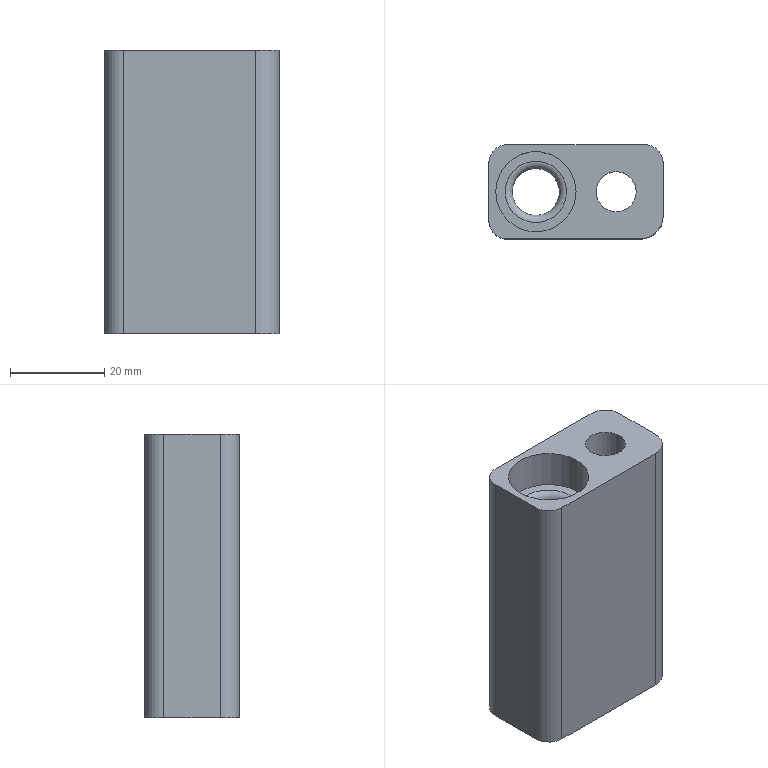Part | STEP file | gslz 2016.10.28-10_id662_x_t | 1 solid | 17 faces | box 37 x 20 x 60 mm | volume 30244 mm3 | plane 8 | cylinder 8 | torus 1 | commonest cylinder face diameters 8 x3 10 x2 8.5 x1 14 x1 17 x1
STEP:
#1=CARTESIAN_POINT('',(0.,0.,0.));
#2=DIRECTION('',(0.,0.,1.));
#3=DIRECTION('',(1.,0.,0.));
#4=AXIS2_PLACEMENT_3D('',#1,#2,#3);
#5=CARTESIAN_POINT('',(1137.841,70.167,85.));
#6=VERTEX_POINT('',#5);
#7=CARTESIAN_POINT('',(1146.341,70.167,85.));
#8=DIRECTION('',(0.,0.,1.));
#9=DIRECTION('',(-1.,0.,0.));
#10=AXIS2_PLACEMENT_3D('',#7,#8,#9);
#11=CIRCLE('',#10,8.5);
#12=CARTESIAN_POINT('',(1105.341,76.167,85.));
#13=DIRECTION('',(0.,0.,1.));
#14=DIRECTION('',(1.,0.,0.));
#15=AXIS2_PLACEMENT_3D('',#12,#13,#14);
#16=PLANE('',#15);
#17=CARTESIAN_POINT('',(41.,-6.));
#18=DIRECTION('',(-1.,0.));
#19=AXIS2_PLACEMENT_2D('',#17,#18);
#20=CIRCLE('',#19,8.5);
#21=(GEOMETRIC_REPRESENTATION_CONTEXT(2)PARAMETRIC_REPRESENTATION_CONTEXT()REPRESENTATION_CONTEXT('',''));
#22=DEFINITIONAL_REPRESENTATION('',(#20),#21);
#23=PCURVE('',#16,#22);
#24=CARTESIAN_POINT('',(1146.341,70.167,81.));
#25=DIRECTION('',(0.,0.,-1.));
#26=DIRECTION('',(1.,0.,0.));
#27=AXIS2_PLACEMENT_3D('',#24,#25,#26);
#28=CYLINDRICAL_SURFACE('',#27,8.5);
#29=CARTESIAN_POINT('',(9.425,-4.));
#30=DIRECTION('',(-1.,0.));
#31=VECTOR('',#30,1.);
#32=LINE('',#29,#31);
#33=(GEOMETRIC_REPRESENTATION_CONTEXT(2)PARAMETRIC_REPRESENTATION_CONTEXT()REPRESENTATION_CONTEXT('',''));
#34=DEFINITIONAL_REPRESENTATION('',(#32),#33);
#35=PCURVE('',#28,#34);
#36=SURFACE_CURVE('',#11,(#23,#35),.PCURVE_S1.);
#37=EDGE_CURVE('',#6,#6,#36,.T.);
#38=ORIENTED_EDGE('',*,*,#37,.F.);
#39=EDGE_LOOP('',(#38));
#40=FACE_BOUND('',#39,.T.);
#41=CARTESIAN_POINT('',(1173.341,65.167,85.));
#42=VERTEX_POINT('',#41);
#43=CARTESIAN_POINT('',(1173.341,76.167,85.));
#44=VERTEX_POINT('',#43);
#45=CARTESIAN_POINT('',(1173.341,76.167,85.));
#46=DIRECTION('',(0.,1.,0.));
#47=VECTOR('',#46,1.);
#48=LINE('',#45,#47);
#49=CARTESIAN_POINT('',(68.,0.));
#50=DIRECTION('',(0.,1.));
#51=VECTOR('',#50,1.);
#52=LINE('',#49,#51);
#53=(GEOMETRIC_REPRESENTATION_CONTEXT(2)PARAMETRIC_REPRESENTATION_CONTEXT()REPRESENTATION_CONTEXT('',''));
#54=DEFINITIONAL_REPRESENTATION('',(#52),#53);
#55=PCURVE('',#16,#54);
#56=CARTESIAN_POINT('',(1173.341,70.167,43.5));
#57=DIRECTION('',(1.,0.,0.));
#58=DIRECTION('',(0.,0.,-1.));
#59=AXIS2_PLACEMENT_3D('',#56,#57,#58);
#60=PLANE('',#59);
#61=CARTESIAN_POINT('',(-41.5,6.));
#62=DIRECTION('',(0.,1.));
#63=VECTOR('',#62,1.);
#64=LINE('',#61,#63);
#65=(GEOMETRIC_REPRESENTATION_CONTEXT(2)PARAMETRIC_REPRESENTATION_CONTEXT()REPRESENTATION_CONTEXT('',''));
#66=DEFINITIONAL_REPRESENTATION('',(#64),#65);
#67=PCURVE('',#60,#66);
#68=SURFACE_CURVE('',#48,(#55,#67),.PCURVE_S1.);
#69=EDGE_CURVE('',#42,#44,#68,.T.);
#70=ORIENTED_EDGE('',*,*,#69,.T.);
#71=CARTESIAN_POINT('',(1169.341,80.167,85.));
#72=VERTEX_POINT('',#71);
#73=CARTESIAN_POINT('',(1169.341,76.167,85.));
#74=DIRECTION('',(0.,0.,1.));
#75=DIRECTION('',(-1.,0.,0.));
#76=AXIS2_PLACEMENT_3D('',#73,#74,#75);
#77=CIRCLE('',#76,4.);
#78=CARTESIAN_POINT('',(64.,0.));
#79=DIRECTION('',(-1.,0.));
#80=AXIS2_PLACEMENT_2D('',#78,#79);
#81=CIRCLE('',#80,4.);
#82=(GEOMETRIC_REPRESENTATION_CONTEXT(2)PARAMETRIC_REPRESENTATION_CONTEXT()REPRESENTATION_CONTEXT('',''));
#83=DEFINITIONAL_REPRESENTATION('',(#81),#82);
#84=PCURVE('',#16,#83);
#85=CARTESIAN_POINT('',(1169.341,76.167,43.5));
#86=DIRECTION('',(0.,0.,-1.));
#87=DIRECTION('',(-1.,0.,0.));
#88=AXIS2_PLACEMENT_3D('',#85,#86,#87);
#89=CYLINDRICAL_SURFACE('',#88,4.);
#90=CARTESIAN_POINT('',(6.283,-41.5));
#91=DIRECTION('',(-1.,0.));
#92=VECTOR('',#91,1.);
#93=LINE('',#90,#92);
#94=(GEOMETRIC_REPRESENTATION_CONTEXT(2)PARAMETRIC_REPRESENTATION_CONTEXT()REPRESENTATION_CONTEXT('',''));
#95=DEFINITIONAL_REPRESENTATION('',(#93),#94);
#96=PCURVE('',#89,#95);
#97=SURFACE_CURVE('',#77,(#84,#96),.PCURVE_S1.);
#98=EDGE_CURVE('',#44,#72,#97,.T.);
#99=ORIENTED_EDGE('',*,*,#98,.T.);
#100=CARTESIAN_POINT('',(1140.341,80.167,85.));
#101=VERTEX_POINT('',#100);
#102=CARTESIAN_POINT('',(1062.706,80.167,85.));
#103=DIRECTION('',(-1.,0.,0.));
#104=VECTOR('',#103,1.);
#105=LINE('',#102,#104);
#106=CARTESIAN_POINT('',(-42.635,4.));
#107=DIRECTION('',(-1.,0.));
#108=VECTOR('',#107,1.);
#109=LINE('',#106,#108);
#110=(GEOMETRIC_REPRESENTATION_CONTEXT(2)PARAMETRIC_REPRESENTATION_CONTEXT()REPRESENTATION_CONTEXT('',''));
#111=DEFINITIONAL_REPRESENTATION('',(#109),#110);
#112=PCURVE('',#16,#111);
#113=CARTESIAN_POINT('',(1062.706,80.167,80.));
#114=DIRECTION('',(0.,-1.,0.));
#115=DIRECTION('',(0.,0.,-1.));
#116=AXIS2_PLACEMENT_3D('',#113,#114,#115);
#117=PLANE('',#116);
#118=CARTESIAN_POINT('',(-5.,0.));
#119=DIRECTION('',(0.,-1.));
#120=VECTOR('',#119,1.);
#121=LINE('',#118,#120);
#122=(GEOMETRIC_REPRESENTATION_CONTEXT(2)PARAMETRIC_REPRESENTATION_CONTEXT()REPRESENTATION_CONTEXT('',''));
#123=DEFINITIONAL_REPRESENTATION('',(#121),#122);
#124=PCURVE('',#117,#123);
#125=SURFACE_CURVE('',#105,(#112,#124),.PCURVE_S1.);
#126=EDGE_CURVE('',#72,#101,#125,.T.);
#127=ORIENTED_EDGE('',*,*,#126,.T.);
#128=CARTESIAN_POINT('',(1136.341,76.167,85.));
#129=VERTEX_POINT('',#128);
#130=CARTESIAN_POINT('',(1140.341,76.167,85.));
#131=DIRECTION('',(0.,0.,1.));
#132=DIRECTION('',(-1.,0.,0.));
#133=AXIS2_PLACEMENT_3D('',#130,#131,#132);
#134=CIRCLE('',#133,4.);
#135=CARTESIAN_POINT('',(35.,0.));
#136=DIRECTION('',(-1.,0.));
#137=AXIS2_PLACEMENT_2D('',#135,#136);
#138=CIRCLE('',#137,4.);
#139=(GEOMETRIC_REPRESENTATION_CONTEXT(2)PARAMETRIC_REPRESENTATION_CONTEXT()REPRESENTATION_CONTEXT('',''));
#140=DEFINITIONAL_REPRESENTATION('',(#138),#139);
#141=PCURVE('',#16,#140);
#142=CARTESIAN_POINT('',(1140.341,76.167,46.));
#143=DIRECTION('',(0.,0.,-1.));
#144=DIRECTION('',(-1.,0.,0.));
#145=AXIS2_PLACEMENT_3D('',#142,#143,#144);
#146=CYLINDRICAL_SURFACE('',#145,4.);
#147=CARTESIAN_POINT('',(6.283,-39.));
#148=DIRECTION('',(-1.,0.));
#149=VECTOR('',#148,1.);
#150=LINE('',#147,#149);
#151=(GEOMETRIC_REPRESENTATION_CONTEXT(2)PARAMETRIC_REPRESENTATION_CONTEXT()REPRESENTATION_CONTEXT('',''));
#152=DEFINITIONAL_REPRESENTATION('',(#150),#151);
#153=PCURVE('',#146,#152);
#154=SURFACE_CURVE('',#134,(#141,#153),.PCURVE_S1.);
#155=EDGE_CURVE('',#101,#129,#154,.T.);
#156=ORIENTED_EDGE('',*,*,#155,.T.);
#157=CARTESIAN_POINT('',(1136.341,64.167,85.));
#158=VERTEX_POINT('',#157);
#159=CARTESIAN_POINT('',(1136.341,70.167,85.));
#160=DIRECTION('',(0.,-1.,0.));
#161=VECTOR('',#160,1.);
#162=LINE('',#159,#161);
#163=CARTESIAN_POINT('',(31.,-6.));
#164=DIRECTION('',(0.,-1.));
#165=VECTOR('',#164,1.);
#166=LINE('',#163,#165);
#167=(GEOMETRIC_REPRESENTATION_CONTEXT(2)PARAMETRIC_REPRESENTATION_CONTEXT()REPRESENTATION_CONTEXT('',''));
#168=DEFINITIONAL_REPRESENTATION('',(#166),#167);
#169=PCURVE('',#16,#168);
#170=CARTESIAN_POINT('',(1136.341,70.167,46.));
#171=DIRECTION('',(1.,0.,0.));
#172=DIRECTION('',(0.,0.,-1.));
#173=AXIS2_PLACEMENT_3D('',#170,#171,#172);
#174=PLANE('',#173);
#175=CARTESIAN_POINT('',(-39.,0.));
#176=DIRECTION('',(0.,-1.));
#177=VECTOR('',#176,1.);
#178=LINE('',#175,#177);
#179=(GEOMETRIC_REPRESENTATION_CONTEXT(2)PARAMETRIC_REPRESENTATION_CONTEXT()REPRESENTATION_CONTEXT('',''));
#180=DEFINITIONAL_REPRESENTATION('',(#178),#179);
#181=PCURVE('',#174,#180);
#182=SURFACE_CURVE('',#162,(#169,#181),.PCURVE_S1.);
#183=EDGE_CURVE('',#129,#158,#182,.T.);
#184=ORIENTED_EDGE('',*,*,#183,.T.);
#185=CARTESIAN_POINT('',(1140.341,60.167,85.));
#186=VERTEX_POINT('',#185);
#187=CARTESIAN_POINT('',(1140.341,64.167,85.));
#188=DIRECTION('',(0.,0.,1.));
#189=DIRECTION('',(-1.,0.,0.));
#190=AXIS2_PLACEMENT_3D('',#187,#188,#189);
#191=CIRCLE('',#190,4.);
#192=CARTESIAN_POINT('',(35.,-12.));
#193=DIRECTION('',(-1.,0.));
#194=AXIS2_PLACEMENT_2D('',#192,#193);
#195=CIRCLE('',#194,4.);
#196=(GEOMETRIC_REPRESENTATION_CONTEXT(2)PARAMETRIC_REPRESENTATION_CONTEXT()REPRESENTATION_CONTEXT('',''));
#197=DEFINITIONAL_REPRESENTATION('',(#195),#196);
#198=PCURVE('',#16,#197);
#199=CARTESIAN_POINT('',(1140.341,64.167,80.));
#200=DIRECTION('',(0.,0.,-1.));
#201=DIRECTION('',(-1.,0.,0.));
#202=AXIS2_PLACEMENT_3D('',#199,#200,#201);
#203=CYLINDRICAL_SURFACE('',#202,4.);
#204=CARTESIAN_POINT('',(6.283,-5.));
#205=DIRECTION('',(-1.,0.));
#206=VECTOR('',#205,1.);
#207=LINE('',#204,#206);
#208=(GEOMETRIC_REPRESENTATION_CONTEXT(2)PARAMETRIC_REPRESENTATION_CONTEXT()REPRESENTATION_CONTEXT('',''));
#209=DEFINITIONAL_REPRESENTATION('',(#207),#208);
#210=PCURVE('',#203,#209);
#211=SURFACE_CURVE('',#191,(#198,#210),.PCURVE_S1.);
#212=EDGE_CURVE('',#158,#186,#211,.T.);
#213=ORIENTED_EDGE('',*,*,#212,.T.);
#214=CARTESIAN_POINT('',(1168.341,60.167,85.));
#215=VERTEX_POINT('',#214);
#216=CARTESIAN_POINT('',(1798.341,60.167,85.));
#217=DIRECTION('',(1.,0.,0.));
#218=VECTOR('',#217,1.);
#219=LINE('',#216,#218);
#220=CARTESIAN_POINT('',(693.,-16.));
#221=DIRECTION('',(1.,0.));
#222=VECTOR('',#221,1.);
#223=LINE('',#220,#222);
#224=(GEOMETRIC_REPRESENTATION_CONTEXT(2)PARAMETRIC_REPRESENTATION_CONTEXT()REPRESENTATION_CONTEXT('',''));
#225=DEFINITIONAL_REPRESENTATION('',(#223),#224);
#226=PCURVE('',#16,#225);
#227=CARTESIAN_POINT('',(1798.341,60.167,80.));
#228=DIRECTION('',(0.,1.,0.));
#229=DIRECTION('',(0.,0.,1.));
#230=AXIS2_PLACEMENT_3D('',#227,#228,#229);
#231=PLANE('',#230);
#232=CARTESIAN_POINT('',(5.,0.));
#233=DIRECTION('',(0.,1.));
#234=VECTOR('',#233,1.);
#235=LINE('',#232,#234);
#236=(GEOMETRIC_REPRESENTATION_CONTEXT(2)PARAMETRIC_REPRESENTATION_CONTEXT()REPRESENTATION_CONTEXT('',''));
#237=DEFINITIONAL_REPRESENTATION('',(#235),#236);
#238=PCURVE('',#231,#237);
#239=SURFACE_CURVE('',#219,(#226,#238),.PCURVE_S1.);
#240=EDGE_CURVE('',#186,#215,#239,.T.);
#241=ORIENTED_EDGE('',*,*,#240,.T.);
#242=CARTESIAN_POINT('',(1168.341,65.167,85.));
#243=DIRECTION('',(0.,0.,1.));
#244=DIRECTION('',(-1.,0.,0.));
#245=AXIS2_PLACEMENT_3D('',#242,#243,#244);
#246=CIRCLE('',#245,5.);
#247=CARTESIAN_POINT('',(63.,-11.));
#248=DIRECTION('',(-1.,0.));
#249=AXIS2_PLACEMENT_2D('',#247,#248);
#250=CIRCLE('',#249,5.);
#251=(GEOMETRIC_REPRESENTATION_CONTEXT(2)PARAMETRIC_REPRESENTATION_CONTEXT()REPRESENTATION_CONTEXT('',''));
#252=DEFINITIONAL_REPRESENTATION('',(#250),#251);
#253=PCURVE('',#16,#252);
#254=CARTESIAN_POINT('',(1168.341,65.167,43.5));
#255=DIRECTION('',(0.,0.,1.));
#256=DIRECTION('',(1.,0.,0.));
#257=AXIS2_PLACEMENT_3D('',#254,#255,#256);
#258=CYLINDRICAL_SURFACE('',#257,5.);
#259=CARTESIAN_POINT('',(3.142,41.5));
#260=DIRECTION('',(1.,0.));
#261=VECTOR('',#260,1.);
#262=LINE('',#259,#261);
#263=(GEOMETRIC_REPRESENTATION_CONTEXT(2)PARAMETRIC_REPRESENTATION_CONTEXT()REPRESENTATION_CONTEXT('',''));
#264=DEFINITIONAL_REPRESENTATION('',(#262),#263);
#265=PCURVE('',#258,#264);
#266=SURFACE_CURVE('',#246,(#253,#265),.PCURVE_S1.);
#267=EDGE_CURVE('',#215,#42,#266,.T.);
#268=ORIENTED_EDGE('',*,*,#267,.T.);
#269=EDGE_LOOP('',(#70,#99,#127,#156,#184,#213,#241,#268));
#270=FACE_BOUND('',#269,.T.);
#271=CARTESIAN_POINT('',(1159.091,70.167,85.));
#272=VERTEX_POINT('',#271);
#273=CARTESIAN_POINT('',(1163.341,70.167,85.));
#274=DIRECTION('',(0.,0.,-1.));
#275=DIRECTION('',(-1.,0.,0.));
#276=AXIS2_PLACEMENT_3D('',#273,#274,#275);
#277=CIRCLE('',#276,4.25);
#278=CARTESIAN_POINT('',(53.75,-6.));
#279=CARTESIAN_POINT('',(53.75,1.361));
#280=CARTESIAN_POINT('',(60.125,-2.319));
#281=CARTESIAN_POINT('',(66.5,-6.));
#282=CARTESIAN_POINT('',(60.125,-9.681));
#283=CARTESIAN_POINT('',(53.75,-13.361));
#284=CARTESIAN_POINT('',(53.75,-6.));
#285=(BOUNDED_CURVE()B_SPLINE_CURVE(2,(#278,#279,#280,#281,#282,#283,#284),.UNSPECIFIED.,.T.,.F.)B_SPLINE_CURVE_WITH_KNOTS((1,2,2,2,2,1),(-2.094,0.,2.094,4.189,6.283,8.378),.UNSPECIFIED.)CURVE()GEOMETRIC_REPRESENTATION_ITEM()RATIONAL_B_SPLINE_CURVE((1.,0.5,1.,0.5,1.,0.5,1.))REPRESENTATION_ITEM(''));
#286=(GEOMETRIC_REPRESENTATION_CONTEXT(2)PARAMETRIC_REPRESENTATION_CONTEXT()REPRESENTATION_CONTEXT('',''));
#287=DEFINITIONAL_REPRESENTATION('',(#285),#286);
#288=PCURVE('',#16,#287);
#289=CARTESIAN_POINT('',(1163.341,70.167,-18.));
#290=DIRECTION('',(0.,0.,1.));
#291=DIRECTION('',(1.,0.,0.));
#292=AXIS2_PLACEMENT_3D('',#289,#290,#291);
#293=CYLINDRICAL_SURFACE('',#292,4.25);
#294=CARTESIAN_POINT('',(9.425,103.));
#295=DIRECTION('',(-1.,0.));
#296=VECTOR('',#295,1.);
#297=LINE('',#294,#296);
#298=(GEOMETRIC_REPRESENTATION_CONTEXT(2)PARAMETRIC_REPRESENTATION_CONTEXT()REPRESENTATION_CONTEXT('',''));
#299=DEFINITIONAL_REPRESENTATION('',(#297),#298);
#300=PCURVE('',#293,#299);
#301=SURFACE_CURVE('',#277,(#288,#300),.PCURVE_S1.);
#302=EDGE_CURVE('',#272,#272,#301,.T.);
#303=ORIENTED_EDGE('',*,*,#302,.T.);
#304=EDGE_LOOP('',(#303));
#305=FACE_BOUND('',#304,.T.);
#306=ADVANCED_FACE('',(#40,#270,#305),#16,.T.);
#307=CARTESIAN_POINT('',(1151.341,70.167,25.));
#308=VERTEX_POINT('',#307);
#309=CARTESIAN_POINT('',(1146.341,70.167,25.));
#310=DIRECTION('',(0.,0.,1.));
#311=DIRECTION('',(1.,0.,0.));
#312=AXIS2_PLACEMENT_3D('',#309,#310,#311);
#313=CIRCLE('',#312,5.);
#314=CARTESIAN_POINT('',(1097.341,16.167,25.));
#315=DIRECTION('',(0.,0.,-1.));
#316=DIRECTION('',(-1.,0.,0.));
#317=AXIS2_PLACEMENT_3D('',#314,#315,#316);
#318=PLANE('',#317);
#319=CARTESIAN_POINT('',(-54.,54.));
#320=CARTESIAN_POINT('',(-54.,62.66));
#321=CARTESIAN_POINT('',(-46.5,58.33));
#322=CARTESIAN_POINT('',(-39.,54.));
#323=CARTESIAN_POINT('',(-46.5,49.67));
#324=CARTESIAN_POINT('',(-54.,45.34));
#325=CARTESIAN_POINT('',(-54.,54.));
#326=(BOUNDED_CURVE()B_SPLINE_CURVE(2,(#319,#320,#321,#322,#323,#324,#325),.UNSPECIFIED.,.T.,.F.)B_SPLINE_CURVE_WITH_KNOTS((1,2,2,2,2,1),(-2.094,0.,2.094,4.189,6.283,8.378),.UNSPECIFIED.)CURVE()GEOMETRIC_REPRESENTATION_ITEM()RATIONAL_B_SPLINE_CURVE((1.,0.5,1.,0.5,1.,0.5,1.))REPRESENTATION_ITEM(''));
#327=(GEOMETRIC_REPRESENTATION_CONTEXT(2)PARAMETRIC_REPRESENTATION_CONTEXT()REPRESENTATION_CONTEXT('',''));
#328=DEFINITIONAL_REPRESENTATION('',(#326),#327);
#329=PCURVE('',#318,#328);
#330=CARTESIAN_POINT('',(1146.341,70.167,45.5));
#331=DIRECTION('',(0.,0.,-1.));
#332=DIRECTION('',(1.,0.,0.));
#333=AXIS2_PLACEMENT_3D('',#330,#331,#332);
#334=CYLINDRICAL_SURFACE('',#333,5.);
#335=CARTESIAN_POINT('',(6.283,20.5));
#336=DIRECTION('',(-1.,0.));
#337=VECTOR('',#336,1.);
#338=LINE('',#335,#337);
#339=(GEOMETRIC_REPRESENTATION_CONTEXT(2)PARAMETRIC_REPRESENTATION_CONTEXT()REPRESENTATION_CONTEXT('',''));
#340=DEFINITIONAL_REPRESENTATION('',(#338),#339);
#341=PCURVE('',#334,#340);
#342=SURFACE_CURVE('',#313,(#329,#341),.PCURVE_S1.);
#343=EDGE_CURVE('',#308,#308,#342,.T.);
#344=ORIENTED_EDGE('',*,*,#343,.T.);
#345=EDGE_LOOP('',(#344));
#346=FACE_BOUND('',#345,.T.);
#347=CARTESIAN_POINT('',(1170.341,70.167,25.));
#348=VERTEX_POINT('',#347);
#349=CARTESIAN_POINT('',(1163.341,70.167,25.));
#350=DIRECTION('',(0.,0.,1.));
#351=DIRECTION('',(1.,0.,0.));
#352=AXIS2_PLACEMENT_3D('',#349,#350,#351);
#353=CIRCLE('',#352,7.);
#354=CARTESIAN_POINT('',(-73.,54.));
#355=CARTESIAN_POINT('',(-73.,66.124));
#356=CARTESIAN_POINT('',(-62.5,60.062));
#357=CARTESIAN_POINT('',(-52.,54.));
#358=CARTESIAN_POINT('',(-62.5,47.938));
#359=CARTESIAN_POINT('',(-73.,41.876));
#360=CARTESIAN_POINT('',(-73.,54.));
#361=(BOUNDED_CURVE()B_SPLINE_CURVE(2,(#354,#355,#356,#357,#358,#359,#360),.UNSPECIFIED.,.T.,.F.)B_SPLINE_CURVE_WITH_KNOTS((1,2,2,2,2,1),(-2.094,0.,2.094,4.189,6.283,8.378),.UNSPECIFIED.)CURVE()GEOMETRIC_REPRESENTATION_ITEM()RATIONAL_B_SPLINE_CURVE((1.,0.5,1.,0.5,1.,0.5,1.))REPRESENTATION_ITEM(''));
#362=(GEOMETRIC_REPRESENTATION_CONTEXT(2)PARAMETRIC_REPRESENTATION_CONTEXT()REPRESENTATION_CONTEXT('',''));
#363=DEFINITIONAL_REPRESENTATION('',(#361),#362);
#364=PCURVE('',#318,#363);
#365=CARTESIAN_POINT('',(1163.341,70.167,-8.));
#366=DIRECTION('',(0.,0.,1.));
#367=DIRECTION('',(1.,0.,0.));
#368=AXIS2_PLACEMENT_3D('',#365,#366,#367);
#369=CYLINDRICAL_SURFACE('',#368,7.);
#370=CARTESIAN_POINT('',(0.,33.));
#371=DIRECTION('',(1.,0.));
#372=VECTOR('',#371,1.);
#373=LINE('',#370,#372);
#374=(GEOMETRIC_REPRESENTATION_CONTEXT(2)PARAMETRIC_REPRESENTATION_CONTEXT()REPRESENTATION_CONTEXT('',''));
#375=DEFINITIONAL_REPRESENTATION('',(#373),#374);
#376=PCURVE('',#369,#375);
#377=SURFACE_CURVE('',#353,(#364,#376),.PCURVE_S1.);
#378=EDGE_CURVE('',#348,#348,#377,.T.);
#379=ORIENTED_EDGE('',*,*,#378,.T.);
#380=EDGE_LOOP('',(#379));
#381=FACE_BOUND('',#380,.T.);
#382=CARTESIAN_POINT('',(1169.341,80.167,25.));
#383=VERTEX_POINT('',#382);
#384=CARTESIAN_POINT('',(1140.341,80.167,25.));
#385=VERTEX_POINT('',#384);
#386=CARTESIAN_POINT('',(1097.341,80.167,25.));
#387=DIRECTION('',(-1.,0.,0.));
#388=VECTOR('',#387,1.);
#389=LINE('',#386,#388);
#390=CARTESIAN_POINT('',(0.,64.));
#391=DIRECTION('',(1.,0.));
#392=VECTOR('',#391,1.);
#393=LINE('',#390,#392);
#394=(GEOMETRIC_REPRESENTATION_CONTEXT(2)PARAMETRIC_REPRESENTATION_CONTEXT()REPRESENTATION_CONTEXT('',''));
#395=DEFINITIONAL_REPRESENTATION('',(#393),#394);
#396=PCURVE('',#318,#395);
#397=CARTESIAN_POINT('',(55.,34.635));
#398=DIRECTION('',(0.,-1.));
#399=VECTOR('',#398,1.);
#400=LINE('',#397,#399);
#401=(GEOMETRIC_REPRESENTATION_CONTEXT(2)PARAMETRIC_REPRESENTATION_CONTEXT()REPRESENTATION_CONTEXT('',''));
#402=DEFINITIONAL_REPRESENTATION('',(#400),#401);
#403=PCURVE('',#117,#402);
#404=SURFACE_CURVE('',#389,(#396,#403),.PCURVE_S1.);
#405=EDGE_CURVE('',#383,#385,#404,.T.);
#406=ORIENTED_EDGE('',*,*,#405,.F.);
#407=CARTESIAN_POINT('',(1173.341,76.167,25.));
#408=VERTEX_POINT('',#407);
#409=CARTESIAN_POINT('',(1169.341,76.167,25.));
#410=DIRECTION('',(0.,0.,-1.));
#411=DIRECTION('',(1.,0.,0.));
#412=AXIS2_PLACEMENT_3D('',#409,#410,#411);
#413=CIRCLE('',#412,4.);
#414=CARTESIAN_POINT('',(-72.,60.));
#415=DIRECTION('',(-1.,0.));
#416=AXIS2_PLACEMENT_2D('',#414,#415);
#417=CIRCLE('',#416,4.);
#418=(GEOMETRIC_REPRESENTATION_CONTEXT(2)PARAMETRIC_REPRESENTATION_CONTEXT()REPRESENTATION_CONTEXT('',''));
#419=DEFINITIONAL_REPRESENTATION('',(#417),#418);
#420=PCURVE('',#318,#419);
#421=CARTESIAN_POINT('',(-3.142,18.5));
#422=DIRECTION('',(1.,0.));
#423=VECTOR('',#422,1.);
#424=LINE('',#421,#423);
#425=(GEOMETRIC_REPRESENTATION_CONTEXT(2)PARAMETRIC_REPRESENTATION_CONTEXT()REPRESENTATION_CONTEXT('',''));
#426=DEFINITIONAL_REPRESENTATION('',(#424),#425);
#427=PCURVE('',#89,#426);
#428=SURFACE_CURVE('',#413,(#420,#427),.PCURVE_S1.);
#429=EDGE_CURVE('',#383,#408,#428,.T.);
#430=ORIENTED_EDGE('',*,*,#429,.T.);
#431=CARTESIAN_POINT('',(1173.341,65.167,25.));
#432=VERTEX_POINT('',#431);
#433=CARTESIAN_POINT('',(1173.341,16.167,25.));
#434=DIRECTION('',(0.,-1.,0.));
#435=VECTOR('',#434,1.);
#436=LINE('',#433,#435);
#437=CARTESIAN_POINT('',(-76.,0.));
#438=DIRECTION('',(0.,-1.));
#439=VECTOR('',#438,1.);
#440=LINE('',#437,#439);
#441=(GEOMETRIC_REPRESENTATION_CONTEXT(2)PARAMETRIC_REPRESENTATION_CONTEXT()REPRESENTATION_CONTEXT('',''));
#442=DEFINITIONAL_REPRESENTATION('',(#440),#441);
#443=PCURVE('',#318,#442);
#444=CARTESIAN_POINT('',(18.5,-54.));
#445=DIRECTION('',(0.,-1.));
#446=VECTOR('',#445,1.);
#447=LINE('',#444,#446);
#448=(GEOMETRIC_REPRESENTATION_CONTEXT(2)PARAMETRIC_REPRESENTATION_CONTEXT()REPRESENTATION_CONTEXT('',''));
#449=DEFINITIONAL_REPRESENTATION('',(#447),#448);
#450=PCURVE('',#60,#449);
#451=SURFACE_CURVE('',#436,(#443,#450),.PCURVE_S1.);
#452=EDGE_CURVE('',#408,#432,#451,.T.);
#453=ORIENTED_EDGE('',*,*,#452,.T.);
#454=CARTESIAN_POINT('',(1168.341,60.167,25.));
#455=VERTEX_POINT('',#454);
#456=CARTESIAN_POINT('',(1168.341,65.167,25.));
#457=DIRECTION('',(0.,0.,-1.));
#458=DIRECTION('',(1.,0.,0.));
#459=AXIS2_PLACEMENT_3D('',#456,#457,#458);
#460=CIRCLE('',#459,5.);
#461=CARTESIAN_POINT('',(-71.,49.));
#462=DIRECTION('',(-1.,0.));
#463=AXIS2_PLACEMENT_2D('',#461,#462);
#464=CIRCLE('',#463,5.);
#465=(GEOMETRIC_REPRESENTATION_CONTEXT(2)PARAMETRIC_REPRESENTATION_CONTEXT()REPRESENTATION_CONTEXT('',''));
#466=DEFINITIONAL_REPRESENTATION('',(#464),#465);
#467=PCURVE('',#318,#466);
#468=CARTESIAN_POINT('',(6.283,-18.5));
#469=DIRECTION('',(-1.,0.));
#470=VECTOR('',#469,1.);
#471=LINE('',#468,#470);
#472=(GEOMETRIC_REPRESENTATION_CONTEXT(2)PARAMETRIC_REPRESENTATION_CONTEXT()REPRESENTATION_CONTEXT('',''));
#473=DEFINITIONAL_REPRESENTATION('',(#471),#472);
#474=PCURVE('',#258,#473);
#475=SURFACE_CURVE('',#460,(#467,#474),.PCURVE_S1.);
#476=EDGE_CURVE('',#432,#455,#475,.T.);
#477=ORIENTED_EDGE('',*,*,#476,.T.);
#478=CARTESIAN_POINT('',(1140.341,60.167,25.));
#479=VERTEX_POINT('',#478);
#480=CARTESIAN_POINT('',(1097.341,60.167,25.));
#481=DIRECTION('',(1.,0.,0.));
#482=VECTOR('',#481,1.);
#483=LINE('',#480,#482);
#484=CARTESIAN_POINT('',(0.,44.));
#485=DIRECTION('',(-1.,0.));
#486=VECTOR('',#485,1.);
#487=LINE('',#484,#486);
#488=(GEOMETRIC_REPRESENTATION_CONTEXT(2)PARAMETRIC_REPRESENTATION_CONTEXT()REPRESENTATION_CONTEXT('',''));
#489=DEFINITIONAL_REPRESENTATION('',(#487),#488);
#490=PCURVE('',#318,#489);
#491=CARTESIAN_POINT('',(-55.,-701.));
#492=DIRECTION('',(0.,1.));
#493=VECTOR('',#492,1.);
#494=LINE('',#491,#493);
#495=(GEOMETRIC_REPRESENTATION_CONTEXT(2)PARAMETRIC_REPRESENTATION_CONTEXT()REPRESENTATION_CONTEXT('',''));
#496=DEFINITIONAL_REPRESENTATION('',(#494),#495);
#497=PCURVE('',#231,#496);
#498=SURFACE_CURVE('',#483,(#490,#497),.PCURVE_S1.);
#499=EDGE_CURVE('',#479,#455,#498,.T.);
#500=ORIENTED_EDGE('',*,*,#499,.F.);
#501=CARTESIAN_POINT('',(1136.341,64.167,25.));
#502=VERTEX_POINT('',#501);
#503=CARTESIAN_POINT('',(1140.341,64.167,25.));
#504=DIRECTION('',(0.,0.,-1.));
#505=DIRECTION('',(1.,0.,0.));
#506=AXIS2_PLACEMENT_3D('',#503,#504,#505);
#507=CIRCLE('',#506,4.);
#508=CARTESIAN_POINT('',(-43.,48.));
#509=DIRECTION('',(-1.,0.));
#510=AXIS2_PLACEMENT_2D('',#508,#509);
#511=CIRCLE('',#510,4.);
#512=(GEOMETRIC_REPRESENTATION_CONTEXT(2)PARAMETRIC_REPRESENTATION_CONTEXT()REPRESENTATION_CONTEXT('',''));
#513=DEFINITIONAL_REPRESENTATION('',(#511),#512);
#514=PCURVE('',#318,#513);
#515=CARTESIAN_POINT('',(3.142,55.));
#516=DIRECTION('',(1.,0.));
#517=VECTOR('',#516,1.);
#518=LINE('',#515,#517);
#519=(GEOMETRIC_REPRESENTATION_CONTEXT(2)PARAMETRIC_REPRESENTATION_CONTEXT()REPRESENTATION_CONTEXT('',''));
#520=DEFINITIONAL_REPRESENTATION('',(#518),#519);
#521=PCURVE('',#203,#520);
#522=SURFACE_CURVE('',#507,(#514,#521),.PCURVE_S1.);
#523=EDGE_CURVE('',#479,#502,#522,.T.);
#524=ORIENTED_EDGE('',*,*,#523,.T.);
#525=CARTESIAN_POINT('',(1136.341,76.167,25.));
#526=VERTEX_POINT('',#525);
#527=CARTESIAN_POINT('',(1136.341,70.167,25.));
#528=DIRECTION('',(0.,1.,0.));
#529=VECTOR('',#528,1.);
#530=LINE('',#527,#529);
#531=CARTESIAN_POINT('',(-39.,54.));
#532=DIRECTION('',(0.,1.));
#533=VECTOR('',#532,1.);
#534=LINE('',#531,#533);
#535=(GEOMETRIC_REPRESENTATION_CONTEXT(2)PARAMETRIC_REPRESENTATION_CONTEXT()REPRESENTATION_CONTEXT('',''));
#536=DEFINITIONAL_REPRESENTATION('',(#534),#535);
#537=PCURVE('',#318,#536);
#538=CARTESIAN_POINT('',(21.,0.));
#539=DIRECTION('',(0.,1.));
#540=VECTOR('',#539,1.);
#541=LINE('',#538,#540);
#542=(GEOMETRIC_REPRESENTATION_CONTEXT(2)PARAMETRIC_REPRESENTATION_CONTEXT()REPRESENTATION_CONTEXT('',''));
#543=DEFINITIONAL_REPRESENTATION('',(#541),#542);
#544=PCURVE('',#174,#543);
#545=SURFACE_CURVE('',#530,(#537,#544),.PCURVE_S1.);
#546=EDGE_CURVE('',#502,#526,#545,.T.);
#547=ORIENTED_EDGE('',*,*,#546,.T.);
#548=CARTESIAN_POINT('',(1140.341,76.167,25.));
#549=DIRECTION('',(0.,0.,-1.));
#550=DIRECTION('',(1.,0.,0.));
#551=AXIS2_PLACEMENT_3D('',#548,#549,#550);
#552=CIRCLE('',#551,4.);
#553=CARTESIAN_POINT('',(-43.,60.));
#554=DIRECTION('',(-1.,0.));
#555=AXIS2_PLACEMENT_2D('',#553,#554);
#556=CIRCLE('',#555,4.);
#557=(GEOMETRIC_REPRESENTATION_CONTEXT(2)PARAMETRIC_REPRESENTATION_CONTEXT()REPRESENTATION_CONTEXT('',''));
#558=DEFINITIONAL_REPRESENTATION('',(#556),#557);
#559=PCURVE('',#318,#558);
#560=CARTESIAN_POINT('',(-3.142,21.));
#561=DIRECTION('',(1.,0.));
#562=VECTOR('',#561,1.);
#563=LINE('',#560,#562);
#564=(GEOMETRIC_REPRESENTATION_CONTEXT(2)PARAMETRIC_REPRESENTATION_CONTEXT()REPRESENTATION_CONTEXT('',''));
#565=DEFINITIONAL_REPRESENTATION('',(#563),#564);
#566=PCURVE('',#146,#565);
#567=SURFACE_CURVE('',#552,(#559,#566),.PCURVE_S1.);
#568=EDGE_CURVE('',#526,#385,#567,.T.);
#569=ORIENTED_EDGE('',*,*,#568,.T.);
#570=EDGE_LOOP('',(#406,#430,#453,#477,#500,#524,#547,#569));
#571=FACE_BOUND('',#570,.T.);
#572=ADVANCED_FACE('',(#346,#381,#571),#318,.T.);
#573=ORIENTED_EDGE('',*,*,#499,.T.);
#574=CARTESIAN_POINT('',(1168.341,60.167,95.));
#575=DIRECTION('',(0.,0.,1.));
#576=VECTOR('',#575,1.);
#577=LINE('',#574,#576);
#578=CARTESIAN_POINT('',(15.,-630.));
#579=DIRECTION('',(1.,0.));
#580=VECTOR('',#579,1.);
#581=LINE('',#578,#580);
#582=(GEOMETRIC_REPRESENTATION_CONTEXT(2)PARAMETRIC_REPRESENTATION_CONTEXT()REPRESENTATION_CONTEXT('',''));
#583=DEFINITIONAL_REPRESENTATION('',(#581),#582);
#584=PCURVE('',#231,#583);
#585=CARTESIAN_POINT('',(4.712,51.5));
#586=DIRECTION('',(0.,1.));
#587=VECTOR('',#586,1.);
#588=LINE('',#585,#587);
#589=(GEOMETRIC_REPRESENTATION_CONTEXT(2)PARAMETRIC_REPRESENTATION_CONTEXT()REPRESENTATION_CONTEXT('',''));
#590=DEFINITIONAL_REPRESENTATION('',(#588),#589);
#591=PCURVE('',#258,#590);
#592=SURFACE_CURVE('',#577,(#584,#591),.PCURVE_S1.);
#593=EDGE_CURVE('',#455,#215,#592,.T.);
#594=ORIENTED_EDGE('',*,*,#593,.T.);
#595=ORIENTED_EDGE('',*,*,#240,.F.);
#596=CARTESIAN_POINT('',(1140.341,60.167,80.));
#597=DIRECTION('',(0.,0.,-1.));
#598=VECTOR('',#597,1.);
#599=LINE('',#596,#598);
#600=CARTESIAN_POINT('',(0.,-658.));
#601=DIRECTION('',(-1.,0.));
#602=VECTOR('',#601,1.);
#603=LINE('',#600,#602);
#604=(GEOMETRIC_REPRESENTATION_CONTEXT(2)PARAMETRIC_REPRESENTATION_CONTEXT()REPRESENTATION_CONTEXT('',''));
#605=DEFINITIONAL_REPRESENTATION('',(#603),#604);
#606=PCURVE('',#231,#605);
#607=CARTESIAN_POINT('',(4.712,0.));
#608=DIRECTION('',(0.,1.));
#609=VECTOR('',#608,1.);
#610=LINE('',#607,#609);
#611=(GEOMETRIC_REPRESENTATION_CONTEXT(2)PARAMETRIC_REPRESENTATION_CONTEXT()REPRESENTATION_CONTEXT('',''));
#612=DEFINITIONAL_REPRESENTATION('',(#610),#611);
#613=PCURVE('',#203,#612);
#614=SURFACE_CURVE('',#599,(#606,#613),.PCURVE_S1.);
#615=EDGE_CURVE('',#186,#479,#614,.T.);
#616=ORIENTED_EDGE('',*,*,#615,.T.);
#617=EDGE_LOOP('',(#573,#594,#595,#616));
#618=FACE_BOUND('',#617,.T.);
#619=ADVANCED_FACE('',(#618),#231,.F.);
#620=ORIENTED_EDGE('',*,*,#126,.F.);
#621=CARTESIAN_POINT('',(1169.341,80.167,43.5));
#622=DIRECTION('',(0.,0.,-1.));
#623=VECTOR('',#622,1.);
#624=LINE('',#621,#623);
#625=CARTESIAN_POINT('',(36.5,106.635));
#626=DIRECTION('',(1.,0.));
#627=VECTOR('',#626,1.);
#628=LINE('',#625,#627);
#629=(GEOMETRIC_REPRESENTATION_CONTEXT(2)PARAMETRIC_REPRESENTATION_CONTEXT()REPRESENTATION_CONTEXT('',''));
#630=DEFINITIONAL_REPRESENTATION('',(#628),#629);
#631=PCURVE('',#117,#630);
#632=CARTESIAN_POINT('',(1.571,0.));
#633=DIRECTION('',(0.,1.));
#634=VECTOR('',#633,1.);
#635=LINE('',#632,#634);
#636=(GEOMETRIC_REPRESENTATION_CONTEXT(2)PARAMETRIC_REPRESENTATION_CONTEXT()REPRESENTATION_CONTEXT('',''));
#637=DEFINITIONAL_REPRESENTATION('',(#635),#636);
#638=PCURVE('',#89,#637);
#639=SURFACE_CURVE('',#624,(#631,#638),.PCURVE_S1.);
#640=EDGE_CURVE('',#72,#383,#639,.T.);
#641=ORIENTED_EDGE('',*,*,#640,.T.);
#642=ORIENTED_EDGE('',*,*,#405,.T.);
#643=CARTESIAN_POINT('',(1140.341,80.167,80.));
#644=DIRECTION('',(0.,0.,1.));
#645=VECTOR('',#644,1.);
#646=LINE('',#643,#645);
#647=CARTESIAN_POINT('',(0.,77.635));
#648=DIRECTION('',(-1.,0.));
#649=VECTOR('',#648,1.);
#650=LINE('',#647,#649);
#651=(GEOMETRIC_REPRESENTATION_CONTEXT(2)PARAMETRIC_REPRESENTATION_CONTEXT()REPRESENTATION_CONTEXT('',''));
#652=DEFINITIONAL_REPRESENTATION('',(#650),#651);
#653=PCURVE('',#117,#652);
#654=CARTESIAN_POINT('',(1.571,-34.));
#655=DIRECTION('',(0.,-1.));
#656=VECTOR('',#655,1.);
#657=LINE('',#654,#656);
#658=(GEOMETRIC_REPRESENTATION_CONTEXT(2)PARAMETRIC_REPRESENTATION_CONTEXT()REPRESENTATION_CONTEXT('',''));
#659=DEFINITIONAL_REPRESENTATION('',(#657),#658);
#660=PCURVE('',#146,#659);
#661=SURFACE_CURVE('',#646,(#653,#660),.PCURVE_S1.);
#662=EDGE_CURVE('',#385,#101,#661,.T.);
#663=ORIENTED_EDGE('',*,*,#662,.T.);
#664=EDGE_LOOP('',(#620,#641,#642,#663));
#665=FACE_BOUND('',#664,.T.);
#666=ADVANCED_FACE('',(#665),#117,.F.);
#667=ORIENTED_EDGE('',*,*,#183,.F.);
#668=CARTESIAN_POINT('',(1136.341,76.167,46.));
#669=DIRECTION('',(0.,0.,-1.));
#670=VECTOR('',#669,1.);
#671=LINE('',#668,#670);
#672=CARTESIAN_POINT('',(0.,6.));
#673=DIRECTION('',(1.,0.));
#674=VECTOR('',#673,1.);
#675=LINE('',#672,#674);
#676=(GEOMETRIC_REPRESENTATION_CONTEXT(2)PARAMETRIC_REPRESENTATION_CONTEXT()REPRESENTATION_CONTEXT('',''));
#677=DEFINITIONAL_REPRESENTATION('',(#675),#676);
#678=PCURVE('',#174,#677);
#679=CARTESIAN_POINT('',(0.,0.));
#680=DIRECTION('',(0.,1.));
#681=VECTOR('',#680,1.);
#682=LINE('',#679,#681);
#683=(GEOMETRIC_REPRESENTATION_CONTEXT(2)PARAMETRIC_REPRESENTATION_CONTEXT()REPRESENTATION_CONTEXT('',''));
#684=DEFINITIONAL_REPRESENTATION('',(#682),#683);
#685=PCURVE('',#146,#684);
#686=SURFACE_CURVE('',#671,(#678,#685),.PCURVE_S1.);
#687=EDGE_CURVE('',#129,#526,#686,.T.);
#688=ORIENTED_EDGE('',*,*,#687,.T.);
#689=ORIENTED_EDGE('',*,*,#546,.F.);
#690=CARTESIAN_POINT('',(1136.341,64.167,46.));
#691=DIRECTION('',(0.,0.,1.));
#692=VECTOR('',#691,1.);
#693=LINE('',#690,#692);
#694=CARTESIAN_POINT('',(0.,-6.));
#695=DIRECTION('',(-1.,0.));
#696=VECTOR('',#695,1.);
#697=LINE('',#694,#696);
#698=(GEOMETRIC_REPRESENTATION_CONTEXT(2)PARAMETRIC_REPRESENTATION_CONTEXT()REPRESENTATION_CONTEXT('',''));
#699=DEFINITIONAL_REPRESENTATION('',(#697),#698);
#700=PCURVE('',#174,#699);
#701=CARTESIAN_POINT('',(6.283,34.));
#702=DIRECTION('',(0.,-1.));
#703=VECTOR('',#702,1.);
#704=LINE('',#701,#703);
#705=(GEOMETRIC_REPRESENTATION_CONTEXT(2)PARAMETRIC_REPRESENTATION_CONTEXT()REPRESENTATION_CONTEXT('',''));
#706=DEFINITIONAL_REPRESENTATION('',(#704),#705);
#707=PCURVE('',#203,#706);
#708=SURFACE_CURVE('',#693,(#700,#707),.PCURVE_S1.);
#709=EDGE_CURVE('',#502,#158,#708,.T.);
#710=ORIENTED_EDGE('',*,*,#709,.T.);
#711=EDGE_LOOP('',(#667,#688,#689,#710));
#712=FACE_BOUND('',#711,.T.);
#713=ADVANCED_FACE('',(#712),#174,.F.);
#714=ORIENTED_EDGE('',*,*,#568,.F.);
#715=ORIENTED_EDGE('',*,*,#687,.F.);
#716=ORIENTED_EDGE('',*,*,#155,.F.);
#717=ORIENTED_EDGE('',*,*,#662,.F.);
#718=EDGE_LOOP('',(#714,#715,#716,#717));
#719=FACE_BOUND('',#718,.T.);
#720=ADVANCED_FACE('',(#719),#146,.T.);
#721=ORIENTED_EDGE('',*,*,#523,.F.);
#722=ORIENTED_EDGE('',*,*,#615,.F.);
#723=ORIENTED_EDGE('',*,*,#212,.F.);
#724=ORIENTED_EDGE('',*,*,#709,.F.);
#725=EDGE_LOOP('',(#721,#722,#723,#724));
#726=FACE_BOUND('',#725,.T.);
#727=ADVANCED_FACE('',(#726),#203,.T.);
#728=CARTESIAN_POINT('',(1159.091,70.167,65.));
#729=VERTEX_POINT('',#728);
#730=CARTESIAN_POINT('',(1163.341,70.167,65.));
#731=DIRECTION('',(0.,0.,1.));
#732=DIRECTION('',(1.,0.,0.));
#733=AXIS2_PLACEMENT_3D('',#730,#731,#732);
#734=CIRCLE('',#733,4.25);
#735=CARTESIAN_POINT('',(0.,83.));
#736=DIRECTION('',(1.,0.));
#737=VECTOR('',#736,1.);
#738=LINE('',#735,#737);
#739=(GEOMETRIC_REPRESENTATION_CONTEXT(2)PARAMETRIC_REPRESENTATION_CONTEXT()REPRESENTATION_CONTEXT('',''));
#740=DEFINITIONAL_REPRESENTATION('',(#738),#739);
#741=PCURVE('',#293,#740);
#742=CARTESIAN_POINT('',(1836.271,152.565,65.));
#743=DIRECTION('',(0.,0.,1.));
#744=DIRECTION('',(1.,0.,0.));
#745=AXIS2_PLACEMENT_3D('',#742,#743,#744);
#746=PLANE('',#745);
#747=CARTESIAN_POINT('',(-672.93,-82.398));
#748=DIRECTION('',(1.,0.));
#749=AXIS2_PLACEMENT_2D('',#747,#748);
#750=CIRCLE('',#749,4.25);
#751=(GEOMETRIC_REPRESENTATION_CONTEXT(2)PARAMETRIC_REPRESENTATION_CONTEXT()REPRESENTATION_CONTEXT('',''));
#752=DEFINITIONAL_REPRESENTATION('',(#750),#751);
#753=PCURVE('',#746,#752);
#754=SURFACE_CURVE('',#734,(#741,#753),.PCURVE_S1.);
#755=EDGE_CURVE('',#729,#729,#754,.T.);
#756=ORIENTED_EDGE('',*,*,#755,.T.);
#757=CARTESIAN_POINT('',(1159.091,70.167,65.));
#758=CARTESIAN_POINT('',(1159.091,70.167,85.));
#759=B_SPLINE_CURVE_WITH_KNOTS('',1,(#757,#758),.UNSPECIFIED.,.F.,.F.,(2,2),(83.,103.),.PIECEWISE_BEZIER_KNOTS.);
#760=CARTESIAN_POINT('',(9.425,0.));
#761=DIRECTION('',(0.,1.));
#762=VECTOR('',#761,1.);
#763=LINE('',#760,#762);
#764=(GEOMETRIC_REPRESENTATION_CONTEXT(2)PARAMETRIC_REPRESENTATION_CONTEXT()REPRESENTATION_CONTEXT('',''));
#765=DEFINITIONAL_REPRESENTATION('',(#763),#764);
#766=PCURVE('',#293,#765);
#767=CARTESIAN_POINT('',(3.142,0.));
#768=DIRECTION('',(0.,1.));
#769=VECTOR('',#768,1.);
#770=LINE('',#767,#769);
#771=(GEOMETRIC_REPRESENTATION_CONTEXT(2)PARAMETRIC_REPRESENTATION_CONTEXT()REPRESENTATION_CONTEXT('',''));
#772=DEFINITIONAL_REPRESENTATION('',(#770),#771);
#773=PCURVE('',#293,#772);
#774=SEAM_CURVE('',#759,(#766,#773),.PCURVE_S1.);
#775=EDGE_CURVE('',#729,#272,#774,.T.);
#776=ORIENTED_EDGE('',*,*,#775,.T.);
#777=ORIENTED_EDGE('',*,*,#302,.T.);
#778=ORIENTED_EDGE('',*,*,#775,.F.);
#779=EDGE_LOOP('',(#756,#776,#777,#778));
#780=FACE_BOUND('',#779,.F.);
#781=ADVANCED_FACE('',(#780),#293,.F.);
#782=ORIENTED_EDGE('',*,*,#755,.T.);
#783=EDGE_LOOP('',(#782));
#784=FACE_BOUND('',#783,.T.);
#785=CARTESIAN_POINT('',(1156.341,70.167,65.));
#786=VERTEX_POINT('',#785);
#787=CARTESIAN_POINT('',(1170.341,70.167,65.));
#788=VERTEX_POINT('',#787);
#789=CARTESIAN_POINT('',(1163.341,70.167,65.));
#790=DIRECTION('',(0.,0.,1.));
#791=DIRECTION('',(1.,0.,0.));
#792=AXIS2_PLACEMENT_3D('',#789,#790,#791);
#793=CIRCLE('',#792,7.);
#794=CARTESIAN_POINT('',(-672.93,-82.398));
#795=DIRECTION('',(1.,0.));
#796=AXIS2_PLACEMENT_2D('',#794,#795);
#797=CIRCLE('',#796,7.);
#798=(GEOMETRIC_REPRESENTATION_CONTEXT(2)PARAMETRIC_REPRESENTATION_CONTEXT()REPRESENTATION_CONTEXT('',''));
#799=DEFINITIONAL_REPRESENTATION('',(#797),#798);
#800=PCURVE('',#746,#799);
#801=CARTESIAN_POINT('',(0.,73.));
#802=DIRECTION('',(1.,0.));
#803=VECTOR('',#802,1.);
#804=LINE('',#801,#803);
#805=(GEOMETRIC_REPRESENTATION_CONTEXT(2)PARAMETRIC_REPRESENTATION_CONTEXT()REPRESENTATION_CONTEXT('',''));
#806=DEFINITIONAL_REPRESENTATION('',(#804),#805);
#807=PCURVE('',#369,#806);
#808=SURFACE_CURVE('',#793,(#800,#807),.PCURVE_S1.);
#809=EDGE_CURVE('',#786,#788,#808,.T.);
#810=ORIENTED_EDGE('',*,*,#809,.F.);
#811=CARTESIAN_POINT('',(1163.341,70.167,65.));
#812=DIRECTION('',(0.,0.,1.));
#813=DIRECTION('',(1.,0.,0.));
#814=AXIS2_PLACEMENT_3D('',#811,#812,#813);
#815=CIRCLE('',#814,7.);
#816=CARTESIAN_POINT('',(-672.93,-82.398));
#817=DIRECTION('',(1.,0.));
#818=AXIS2_PLACEMENT_2D('',#816,#817);
#819=CIRCLE('',#818,7.);
#820=(GEOMETRIC_REPRESENTATION_CONTEXT(2)PARAMETRIC_REPRESENTATION_CONTEXT()REPRESENTATION_CONTEXT('',''));
#821=DEFINITIONAL_REPRESENTATION('',(#819),#820);
#822=PCURVE('',#746,#821);
#823=CARTESIAN_POINT('',(-6.283,73.));
#824=DIRECTION('',(1.,0.));
#825=VECTOR('',#824,1.);
#826=LINE('',#823,#825);
#827=(GEOMETRIC_REPRESENTATION_CONTEXT(2)PARAMETRIC_REPRESENTATION_CONTEXT()REPRESENTATION_CONTEXT('',''));
#828=DEFINITIONAL_REPRESENTATION('',(#826),#827);
#829=PCURVE('',#369,#828);
#830=SURFACE_CURVE('',#815,(#822,#829),.PCURVE_S1.);
#831=EDGE_CURVE('',#788,#786,#830,.T.);
#832=ORIENTED_EDGE('',*,*,#831,.F.);
#833=EDGE_LOOP('',(#810,#832));
#834=FACE_BOUND('',#833,.T.);
#835=ADVANCED_FACE('',(#784,#834),#746,.F.);
#836=ORIENTED_EDGE('',*,*,#831,.F.);
#837=CARTESIAN_POINT('',(1170.341,70.167,25.));
#838=CARTESIAN_POINT('',(1170.341,70.167,65.));
#839=B_SPLINE_CURVE_WITH_KNOTS('',1,(#837,#838),.UNSPECIFIED.,.F.,.F.,(2,2),(33.,73.),.PIECEWISE_BEZIER_KNOTS.);
#840=CARTESIAN_POINT('',(0.,0.));
#841=DIRECTION('',(0.,1.));
#842=VECTOR('',#841,1.);
#843=LINE('',#840,#842);
#844=(GEOMETRIC_REPRESENTATION_CONTEXT(2)PARAMETRIC_REPRESENTATION_CONTEXT()REPRESENTATION_CONTEXT('',''));
#845=DEFINITIONAL_REPRESENTATION('',(#843),#844);
#846=PCURVE('',#369,#845);
#847=CARTESIAN_POINT('',(6.283,0.));
#848=DIRECTION('',(0.,1.));
#849=VECTOR('',#848,1.);
#850=LINE('',#847,#849);
#851=(GEOMETRIC_REPRESENTATION_CONTEXT(2)PARAMETRIC_REPRESENTATION_CONTEXT()REPRESENTATION_CONTEXT('',''));
#852=DEFINITIONAL_REPRESENTATION('',(#850),#851);
#853=PCURVE('',#369,#852);
#854=SEAM_CURVE('',#839,(#846,#853),.PCURVE_S1.);
#855=EDGE_CURVE('',#348,#788,#854,.T.);
#856=ORIENTED_EDGE('',*,*,#855,.F.);
#857=ORIENTED_EDGE('',*,*,#378,.T.);
#858=ORIENTED_EDGE('',*,*,#855,.T.);
#859=ORIENTED_EDGE('',*,*,#809,.F.);
#860=EDGE_LOOP('',(#836,#856,#857,#858,#859));
#861=FACE_BOUND('',#860,.F.);
#862=ADVANCED_FACE('',(#861),#369,.F.);
#863=ORIENTED_EDGE('',*,*,#452,.F.);
#864=CARTESIAN_POINT('',(1173.341,76.167,43.5));
#865=DIRECTION('',(0.,0.,1.));
#866=VECTOR('',#865,1.);
#867=LINE('',#864,#866);
#868=CARTESIAN_POINT('',(0.,6.));
#869=DIRECTION('',(-1.,0.));
#870=VECTOR('',#869,1.);
#871=LINE('',#868,#870);
#872=(GEOMETRIC_REPRESENTATION_CONTEXT(2)PARAMETRIC_REPRESENTATION_CONTEXT()REPRESENTATION_CONTEXT('',''));
#873=DEFINITIONAL_REPRESENTATION('',(#871),#872);
#874=PCURVE('',#60,#873);
#875=CARTESIAN_POINT('',(3.142,0.));
#876=DIRECTION('',(0.,-1.));
#877=VECTOR('',#876,1.);
#878=LINE('',#875,#877);
#879=(GEOMETRIC_REPRESENTATION_CONTEXT(2)PARAMETRIC_REPRESENTATION_CONTEXT()REPRESENTATION_CONTEXT('',''));
#880=DEFINITIONAL_REPRESENTATION('',(#878),#879);
#881=PCURVE('',#89,#880);
#882=SURFACE_CURVE('',#867,(#874,#881),.PCURVE_S1.);
#883=EDGE_CURVE('',#408,#44,#882,.T.);
#884=ORIENTED_EDGE('',*,*,#883,.T.);
#885=ORIENTED_EDGE('',*,*,#69,.F.);
#886=CARTESIAN_POINT('',(1173.341,65.167,45.));
#887=DIRECTION('',(0.,0.,-1.));
#888=VECTOR('',#887,1.);
#889=LINE('',#886,#888);
#890=CARTESIAN_POINT('',(-1.5,-5.));
#891=DIRECTION('',(1.,0.));
#892=VECTOR('',#891,1.);
#893=LINE('',#890,#892);
#894=(GEOMETRIC_REPRESENTATION_CONTEXT(2)PARAMETRIC_REPRESENTATION_CONTEXT()REPRESENTATION_CONTEXT('',''));
#895=DEFINITIONAL_REPRESENTATION('',(#893),#894);
#896=PCURVE('',#60,#895);
#897=CARTESIAN_POINT('',(6.283,1.5));
#898=DIRECTION('',(0.,-1.));
#899=VECTOR('',#898,1.);
#900=LINE('',#897,#899);
#901=(GEOMETRIC_REPRESENTATION_CONTEXT(2)PARAMETRIC_REPRESENTATION_CONTEXT()REPRESENTATION_CONTEXT('',''));
#902=DEFINITIONAL_REPRESENTATION('',(#900),#901);
#903=PCURVE('',#258,#902);
#904=SURFACE_CURVE('',#889,(#896,#903),.PCURVE_S1.);
#905=EDGE_CURVE('',#42,#432,#904,.T.);
#906=ORIENTED_EDGE('',*,*,#905,.T.);
#907=EDGE_LOOP('',(#863,#884,#885,#906));
#908=FACE_BOUND('',#907,.T.);
#909=ADVANCED_FACE('',(#908),#60,.T.);
#910=CARTESIAN_POINT('',(1141.341,70.167,75.45));
#911=VERTEX_POINT('',#910);
#912=CARTESIAN_POINT('',(1151.341,70.167,75.45));
#913=VERTEX_POINT('',#912);
#914=CARTESIAN_POINT('',(1146.341,70.167,75.45));
#915=DIRECTION('',(0.,0.,-1.));
#916=DIRECTION('',(-1.,0.,0.));
#917=AXIS2_PLACEMENT_3D('',#914,#915,#916);
#918=CIRCLE('',#917,5.);
#919=CARTESIAN_POINT('',(3.142,-29.95));
#920=DIRECTION('',(1.,0.));
#921=VECTOR('',#920,1.);
#922=LINE('',#919,#921);
#923=(GEOMETRIC_REPRESENTATION_CONTEXT(2)PARAMETRIC_REPRESENTATION_CONTEXT()REPRESENTATION_CONTEXT('',''));
#924=DEFINITIONAL_REPRESENTATION('',(#922),#923);
#925=PCURVE('',#334,#924);
#926=CARTESIAN_POINT('',(1146.341,70.167,75.45));
#927=DIRECTION('',(0.,0.,1.));
#928=DIRECTION('',(1.,0.,0.));
#929=AXIS2_PLACEMENT_3D('',#926,#927,#928);
#930=TOROIDAL_SURFACE('',#929,6.5,1.5);
#931=CARTESIAN_POINT('',(9.425,9.425));
#932=DIRECTION('',(-1.,0.));
#933=VECTOR('',#932,1.);
#934=LINE('',#931,#933);
#935=(GEOMETRIC_REPRESENTATION_CONTEXT(2)PARAMETRIC_REPRESENTATION_CONTEXT()REPRESENTATION_CONTEXT('',''));
#936=DEFINITIONAL_REPRESENTATION('',(#934),#935);
#937=PCURVE('',#930,#936);
#938=SURFACE_CURVE('',#918,(#925,#937),.PCURVE_S1.);
#939=EDGE_CURVE('',#911,#913,#938,.T.);
#940=ORIENTED_EDGE('',*,*,#939,.T.);
#941=CARTESIAN_POINT('',(1151.341,70.167,75.45));
#942=CARTESIAN_POINT('',(1151.341,70.167,25.));
#943=B_SPLINE_CURVE_WITH_KNOTS('',1,(#941,#942),.UNSPECIFIED.,.F.,.F.,(2,2),(-29.95,20.5),.PIECEWISE_BEZIER_KNOTS.);
#944=CARTESIAN_POINT('',(6.283,0.));
#945=DIRECTION('',(0.,1.));
#946=VECTOR('',#945,1.);
#947=LINE('',#944,#946);
#948=(GEOMETRIC_REPRESENTATION_CONTEXT(2)PARAMETRIC_REPRESENTATION_CONTEXT()REPRESENTATION_CONTEXT('',''));
#949=DEFINITIONAL_REPRESENTATION('',(#947),#948);
#950=PCURVE('',#334,#949);
#951=CARTESIAN_POINT('',(0.,0.));
#952=DIRECTION('',(0.,1.));
#953=VECTOR('',#952,1.);
#954=LINE('',#951,#953);
#955=(GEOMETRIC_REPRESENTATION_CONTEXT(2)PARAMETRIC_REPRESENTATION_CONTEXT()REPRESENTATION_CONTEXT('',''));
#956=DEFINITIONAL_REPRESENTATION('',(#954),#955);
#957=PCURVE('',#334,#956);
#958=SEAM_CURVE('',#943,(#950,#957),.PCURVE_S1.);
#959=EDGE_CURVE('',#913,#308,#958,.T.);
#960=ORIENTED_EDGE('',*,*,#959,.T.);
#961=ORIENTED_EDGE('',*,*,#343,.T.);
#962=ORIENTED_EDGE('',*,*,#959,.F.);
#963=CARTESIAN_POINT('',(1146.341,70.167,75.45));
#964=DIRECTION('',(0.,0.,-1.));
#965=DIRECTION('',(-1.,0.,0.));
#966=AXIS2_PLACEMENT_3D('',#963,#964,#965);
#967=CIRCLE('',#966,5.);
#968=CARTESIAN_POINT('',(-3.142,-29.95));
#969=DIRECTION('',(1.,0.));
#970=VECTOR('',#969,1.);
#971=LINE('',#968,#970);
#972=(GEOMETRIC_REPRESENTATION_CONTEXT(2)PARAMETRIC_REPRESENTATION_CONTEXT()REPRESENTATION_CONTEXT('',''));
#973=DEFINITIONAL_REPRESENTATION('',(#971),#972);
#974=PCURVE('',#334,#973);
#975=CARTESIAN_POINT('',(9.425,9.425));
#976=DIRECTION('',(-1.,0.));
#977=VECTOR('',#976,1.);
#978=LINE('',#975,#977);
#979=(GEOMETRIC_REPRESENTATION_CONTEXT(2)PARAMETRIC_REPRESENTATION_CONTEXT()REPRESENTATION_CONTEXT('',''));
#980=DEFINITIONAL_REPRESENTATION('',(#978),#979);
#981=PCURVE('',#930,#980);
#982=SURFACE_CURVE('',#967,(#974,#981),.PCURVE_S1.);
#983=EDGE_CURVE('',#913,#911,#982,.T.);
#984=ORIENTED_EDGE('',*,*,#983,.T.);
#985=EDGE_LOOP('',(#940,#960,#961,#962,#984));
#986=FACE_BOUND('',#985,.F.);
#987=ADVANCED_FACE('',(#986),#334,.F.);
#988=CARTESIAN_POINT('',(1137.841,70.167,76.95));
#989=VERTEX_POINT('',#988);
#990=CARTESIAN_POINT('',(1146.341,70.167,76.95));
#991=DIRECTION('',(0.,0.,1.));
#992=DIRECTION('',(-1.,0.,0.));
#993=AXIS2_PLACEMENT_3D('',#990,#991,#992);
#994=CIRCLE('',#993,8.5);
#995=CARTESIAN_POINT('',(9.425,4.05));
#996=DIRECTION('',(-1.,0.));
#997=VECTOR('',#996,1.);
#998=LINE('',#995,#997);
#999=(GEOMETRIC_REPRESENTATION_CONTEXT(2)PARAMETRIC_REPRESENTATION_CONTEXT()REPRESENTATION_CONTEXT('',''));
#1000=DEFINITIONAL_REPRESENTATION('',(#998),#999);
#1001=PCURVE('',#28,#1000);
#1002=CARTESIAN_POINT('',(1105.341,76.167,76.95));
#1003=DIRECTION('',(0.,0.,1.));
#1004=DIRECTION('',(1.,0.,0.));
#1005=AXIS2_PLACEMENT_3D('',#1002,#1003,#1004);
#1006=PLANE('',#1005);
#1007=CARTESIAN_POINT('',(41.,-6.));
#1008=DIRECTION('',(-1.,0.));
#1009=AXIS2_PLACEMENT_2D('',#1007,#1008);
#1010=CIRCLE('',#1009,8.5);
#1011=(GEOMETRIC_REPRESENTATION_CONTEXT(2)PARAMETRIC_REPRESENTATION_CONTEXT()REPRESENTATION_CONTEXT('',''));
#1012=DEFINITIONAL_REPRESENTATION('',(#1010),#1011);
#1013=PCURVE('',#1006,#1012);
#1014=SURFACE_CURVE('',#994,(#1001,#1013),.PCURVE_S1.);
#1015=EDGE_CURVE('',#989,#989,#1014,.T.);
#1016=ORIENTED_EDGE('',*,*,#1015,.T.);
#1017=CARTESIAN_POINT('',(1137.841,70.167,85.));
#1018=CARTESIAN_POINT('',(1137.841,70.167,76.95));
#1019=B_SPLINE_CURVE_WITH_KNOTS('',1,(#1017,#1018),.UNSPECIFIED.,.F.,.F.,(2,2),(-4.,4.05),.PIECEWISE_BEZIER_KNOTS.);
#1020=CARTESIAN_POINT('',(3.142,0.));
#1021=DIRECTION('',(0.,1.));
#1022=VECTOR('',#1021,1.);
#1023=LINE('',#1020,#1022);
#1024=(GEOMETRIC_REPRESENTATION_CONTEXT(2)PARAMETRIC_REPRESENTATION_CONTEXT()REPRESENTATION_CONTEXT('',''));
#1025=DEFINITIONAL_REPRESENTATION('',(#1023),#1024);
#1026=PCURVE('',#28,#1025);
#1027=CARTESIAN_POINT('',(9.425,0.));
#1028=DIRECTION('',(0.,1.));
#1029=VECTOR('',#1028,1.);
#1030=LINE('',#1027,#1029);
#1031=(GEOMETRIC_REPRESENTATION_CONTEXT(2)PARAMETRIC_REPRESENTATION_CONTEXT()REPRESENTATION_CONTEXT('',''));
#1032=DEFINITIONAL_REPRESENTATION('',(#1030),#1031);
#1033=PCURVE('',#28,#1032);
#1034=SEAM_CURVE('',#1019,(#1026,#1033),.PCURVE_S1.);
#1035=EDGE_CURVE('',#6,#989,#1034,.T.);
#1036=ORIENTED_EDGE('',*,*,#1035,.F.);
#1037=ORIENTED_EDGE('',*,*,#37,.F.);
#1038=ORIENTED_EDGE('',*,*,#1035,.T.);
#1039=EDGE_LOOP('',(#1016,#1036,#1037,#1038));
#1040=FACE_BOUND('',#1039,.F.);
#1041=ADVANCED_FACE('',(#1040),#28,.F.);
#1042=ORIENTED_EDGE('',*,*,#939,.T.);
#1043=ORIENTED_EDGE('',*,*,#983,.T.);
#1044=CARTESIAN_POINT('',(1139.841,70.167,76.95));
#1045=VERTEX_POINT('',#1044);
#1046=CARTESIAN_POINT('',(1139.841,70.167,76.95));
#1047=CARTESIAN_POINT('',(1140.242,70.167,76.95));
#1048=CARTESIAN_POINT('',(1140.632,70.167,76.822));
#1049=CARTESIAN_POINT('',(1140.969,70.167,76.578));
#1050=CARTESIAN_POINT('',(1141.213,70.167,76.242));
#1051=CARTESIAN_POINT('',(1141.341,70.167,75.851));
#1052=CARTESIAN_POINT('',(1141.341,70.167,75.45));
#1053=(BOUNDED_CURVE()B_SPLINE_CURVE(6,(#1046,#1047,#1048,#1049,#1050,#1051,#1052),.UNSPECIFIED.,.F.,.F.)B_SPLINE_CURVE_WITH_KNOTS((7,7),(1.571,3.142),.PIECEWISE_BEZIER_KNOTS.)CURVE()GEOMETRIC_REPRESENTATION_ITEM()RATIONAL_B_SPLINE_CURVE((1.031,1.01,0.9979,0.994,0.9979,1.01,1.031))REPRESENTATION_ITEM(''));
#1054=CARTESIAN_POINT('',(3.142,6.283));
#1055=DIRECTION('',(0.,1.));
#1056=VECTOR('',#1055,1.);
#1057=LINE('',#1054,#1056);
#1058=(GEOMETRIC_REPRESENTATION_CONTEXT(2)PARAMETRIC_REPRESENTATION_CONTEXT()REPRESENTATION_CONTEXT('',''));
#1059=DEFINITIONAL_REPRESENTATION('',(#1057),#1058);
#1060=PCURVE('',#930,#1059);
#1061=CARTESIAN_POINT('',(9.425,6.283));
#1062=DIRECTION('',(0.,1.));
#1063=VECTOR('',#1062,1.);
#1064=LINE('',#1061,#1063);
#1065=(GEOMETRIC_REPRESENTATION_CONTEXT(2)PARAMETRIC_REPRESENTATION_CONTEXT()REPRESENTATION_CONTEXT('',''));
#1066=DEFINITIONAL_REPRESENTATION('',(#1064),#1065);
#1067=PCURVE('',#930,#1066);
#1068=SEAM_CURVE('',#1053,(#1060,#1067),.PCURVE_S1.);
#1069=EDGE_CURVE('',#1045,#911,#1068,.T.);
#1070=ORIENTED_EDGE('',*,*,#1069,.F.);
#1071=CARTESIAN_POINT('',(1146.341,70.167,76.95));
#1072=DIRECTION('',(0.,0.,1.));
#1073=DIRECTION('',(-1.,0.,0.));
#1074=AXIS2_PLACEMENT_3D('',#1071,#1072,#1073);
#1075=CIRCLE('',#1074,6.5);
#1076=CARTESIAN_POINT('',(3.142,7.854));
#1077=DIRECTION('',(1.,0.));
#1078=VECTOR('',#1077,1.);
#1079=LINE('',#1076,#1078);
#1080=(GEOMETRIC_REPRESENTATION_CONTEXT(2)PARAMETRIC_REPRESENTATION_CONTEXT()REPRESENTATION_CONTEXT('',''));
#1081=DEFINITIONAL_REPRESENTATION('',(#1079),#1080);
#1082=PCURVE('',#930,#1081);
#1083=CARTESIAN_POINT('',(41.,-6.));
#1084=DIRECTION('',(-1.,0.));
#1085=AXIS2_PLACEMENT_2D('',#1083,#1084);
#1086=CIRCLE('',#1085,6.5);
#1087=(GEOMETRIC_REPRESENTATION_CONTEXT(2)PARAMETRIC_REPRESENTATION_CONTEXT()REPRESENTATION_CONTEXT('',''));
#1088=DEFINITIONAL_REPRESENTATION('',(#1086),#1087);
#1089=PCURVE('',#1006,#1088);
#1090=SURFACE_CURVE('',#1075,(#1082,#1089),.PCURVE_S1.);
#1091=EDGE_CURVE('',#1045,#1045,#1090,.T.);
#1092=ORIENTED_EDGE('',*,*,#1091,.T.);
#1093=ORIENTED_EDGE('',*,*,#1069,.T.);
#1094=EDGE_LOOP('',(#1042,#1043,#1070,#1092,#1093));
#1095=FACE_BOUND('',#1094,.T.);
#1096=ADVANCED_FACE('',(#1095),#930,.T.);
#1097=ORIENTED_EDGE('',*,*,#1015,.T.);
#1098=EDGE_LOOP('',(#1097));
#1099=FACE_BOUND('',#1098,.T.);
#1100=ORIENTED_EDGE('',*,*,#1091,.F.);
#1101=EDGE_LOOP('',(#1100));
#1102=FACE_BOUND('',#1101,.T.);
#1103=ADVANCED_FACE('',(#1099,#1102),#1006,.T.);
#1104=ORIENTED_EDGE('',*,*,#267,.F.);
#1105=ORIENTED_EDGE('',*,*,#593,.F.);
#1106=ORIENTED_EDGE('',*,*,#476,.F.);
#1107=ORIENTED_EDGE('',*,*,#905,.F.);
#1108=EDGE_LOOP('',(#1104,#1105,#1106,#1107));
#1109=FACE_BOUND('',#1108,.T.);
#1110=ADVANCED_FACE('',(#1109),#258,.T.);
#1111=ORIENTED_EDGE('',*,*,#98,.F.);
#1112=ORIENTED_EDGE('',*,*,#883,.F.);
#1113=ORIENTED_EDGE('',*,*,#429,.F.);
#1114=ORIENTED_EDGE('',*,*,#640,.F.);
#1115=EDGE_LOOP('',(#1111,#1112,#1113,#1114));
#1116=FACE_BOUND('',#1115,.T.);
#1117=ADVANCED_FACE('',(#1116),#89,.T.);
#1118=CLOSED_SHELL('',(#306,#572,#619,#666,#713,#720,#727,#781,#835,#862,#909,#987,#1041,#1096,#1103,#1110,#1117));
#1119=MANIFOLD_SOLID_BREP('',#1118);
#1120=(LENGTH_UNIT()NAMED_UNIT(*)SI_UNIT(.MILLI.,.METRE.));
#1121=UNCERTAINTY_MEASURE_WITH_UNIT(LENGTH_MEASURE(0.000002),#1120,'','');
#1122=(NAMED_UNIT(*)PLANE_ANGLE_UNIT()SI_UNIT($,.RADIAN.));
#1123=(NAMED_UNIT(*)SI_UNIT($,.STERADIAN.)SOLID_ANGLE_UNIT());
#1124=(GEOMETRIC_REPRESENTATION_CONTEXT(3)GLOBAL_UNCERTAINTY_ASSIGNED_CONTEXT((#1121))GLOBAL_UNIT_ASSIGNED_CONTEXT((#1120,#1122,#1123))REPRESENTATION_CONTEXT('',''));
#1125=ADVANCED_BREP_SHAPE_REPRESENTATION('',(#4,#1119),#1124);